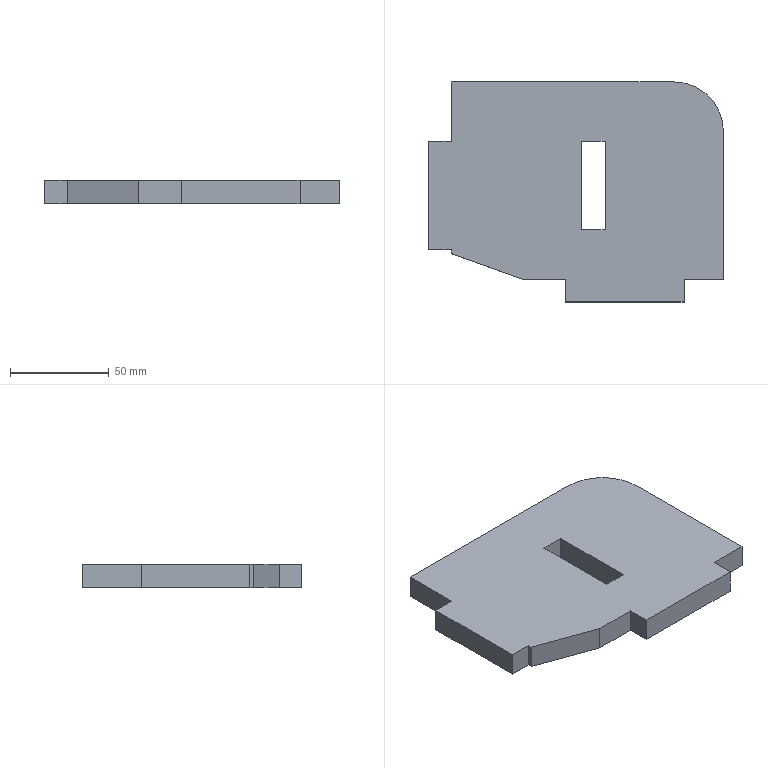Part | SolidWorks | features FlatPattern 1, SMBaseFlange 1, SheetMetal 1 | 1 solid | 20 faces | box 149.5 x 111.5 x 12 mm | volume 170572 mm3 | plane 19 | cylinder 1 | commonest cylinder face diameters 50 x1
STEP:
#1=CARTESIAN_POINT('',(382.937,67.282,0.));
#2=VERTEX_POINT('',#1);
#3=CARTESIAN_POINT('',(382.937,142.282,0.));
#4=VERTEX_POINT('',#3);
#5=CARTESIAN_POINT('',(382.937,67.282,0.));
#6=DIRECTION('',(0.,1.,0.));
#7=VECTOR('',#6,1000.);
#8=LINE('',#5,#7);
#9=EDGE_CURVE('',#2,#4,#8,.T.);
#10=ORIENTED_EDGE('',*,*,#9,.F.);
#11=CARTESIAN_POINT('',(382.937,67.282,-12.));
#12=VERTEX_POINT('',#11);
#13=CARTESIAN_POINT('',(382.937,67.282,-12.));
#14=DIRECTION('',(0.,0.,1.));
#15=VECTOR('',#14,1000.);
#16=LINE('',#13,#15);
#17=EDGE_CURVE('',#12,#2,#16,.T.);
#18=ORIENTED_EDGE('',*,*,#17,.F.);
#19=CARTESIAN_POINT('',(382.937,142.282,-12.));
#20=VERTEX_POINT('',#19);
#21=CARTESIAN_POINT('',(382.937,67.282,-12.));
#22=DIRECTION('',(0.,1.,0.));
#23=VECTOR('',#22,1000.);
#24=LINE('',#21,#23);
#25=EDGE_CURVE('',#12,#20,#24,.T.);
#26=ORIENTED_EDGE('',*,*,#25,.T.);
#27=CARTESIAN_POINT('',(382.937,142.282,-12.));
#28=DIRECTION('',(0.,0.,1.));
#29=VECTOR('',#28,1000.);
#30=LINE('',#27,#29);
#31=EDGE_CURVE('',#20,#4,#30,.T.);
#32=ORIENTED_EDGE('',*,*,#31,.T.);
#33=EDGE_LOOP('',(#10,#18,#26,#32));
#34=FACE_OUTER_BOUND('',#33,.T.);
#35=CARTESIAN_POINT('',(382.937,67.282,-12.));
#36=DIRECTION('',(1.,0.,0.));
#37=DIRECTION('',(0.,0.,-1.));
#38=AXIS2_PLACEMENT_3D('',#35,#36,#37);
#39=PLANE('',#38);
#40=ADVANCED_FACE('',(#34),#39,.T.);
#41=CARTESIAN_POINT('',(362.937,67.282,0.));
#42=VERTEX_POINT('',#41);
#43=CARTESIAN_POINT('',(382.937,67.282,0.));
#44=DIRECTION('',(1.,0.,0.));
#45=VECTOR('',#44,1000.);
#46=LINE('',#43,#45);
#47=EDGE_CURVE('',#42,#2,#46,.T.);
#48=ORIENTED_EDGE('',*,*,#47,.F.);
#49=CARTESIAN_POINT('',(362.937,67.282,-12.));
#50=VERTEX_POINT('',#49);
#51=CARTESIAN_POINT('',(362.937,67.282,-12.));
#52=DIRECTION('',(0.,0.,1.));
#53=VECTOR('',#52,1000.);
#54=LINE('',#51,#53);
#55=EDGE_CURVE('',#50,#42,#54,.T.);
#56=ORIENTED_EDGE('',*,*,#55,.F.);
#57=CARTESIAN_POINT('',(382.937,67.282,-12.));
#58=DIRECTION('',(1.,0.,0.));
#59=VECTOR('',#58,1000.);
#60=LINE('',#57,#59);
#61=EDGE_CURVE('',#50,#12,#60,.T.);
#62=ORIENTED_EDGE('',*,*,#61,.T.);
#63=ORIENTED_EDGE('',*,*,#17,.T.);
#64=EDGE_LOOP('',(#48,#56,#62,#63));
#65=FACE_OUTER_BOUND('',#64,.T.);
#66=CARTESIAN_POINT('',(382.937,67.282,-12.));
#67=DIRECTION('',(0.,-1.,0.));
#68=DIRECTION('',(0.,0.,-1.));
#69=AXIS2_PLACEMENT_3D('',#66,#67,#68);
#70=PLANE('',#69);
#71=ADVANCED_FACE('',(#65),#70,.T.);
#72=CARTESIAN_POINT('',(362.937,55.782,0.));
#73=VERTEX_POINT('',#72);
#74=CARTESIAN_POINT('',(362.937,55.782,0.));
#75=DIRECTION('',(0.,1.,0.));
#76=VECTOR('',#75,1000.);
#77=LINE('',#74,#76);
#78=EDGE_CURVE('',#73,#42,#77,.T.);
#79=ORIENTED_EDGE('',*,*,#78,.F.);
#80=CARTESIAN_POINT('',(362.937,55.782,-12.));
#81=VERTEX_POINT('',#80);
#82=CARTESIAN_POINT('',(362.937,55.782,-12.));
#83=DIRECTION('',(0.,0.,1.));
#84=VECTOR('',#83,1000.);
#85=LINE('',#82,#84);
#86=EDGE_CURVE('',#81,#73,#85,.T.);
#87=ORIENTED_EDGE('',*,*,#86,.F.);
#88=CARTESIAN_POINT('',(362.937,55.782,-12.));
#89=DIRECTION('',(0.,1.,0.));
#90=VECTOR('',#89,1000.);
#91=LINE('',#88,#90);
#92=EDGE_CURVE('',#81,#50,#91,.T.);
#93=ORIENTED_EDGE('',*,*,#92,.T.);
#94=ORIENTED_EDGE('',*,*,#55,.T.);
#95=EDGE_LOOP('',(#79,#87,#93,#94));
#96=FACE_OUTER_BOUND('',#95,.T.);
#97=CARTESIAN_POINT('',(362.937,55.782,-12.));
#98=DIRECTION('',(1.,0.,0.));
#99=DIRECTION('',(0.,0.,-1.));
#100=AXIS2_PLACEMENT_3D('',#97,#98,#99);
#101=PLANE('',#100);
#102=ADVANCED_FACE('',(#96),#101,.T.);
#103=CARTESIAN_POINT('',(302.937,55.782,0.));
#104=VERTEX_POINT('',#103);
#105=CARTESIAN_POINT('',(302.937,55.782,0.));
#106=DIRECTION('',(1.,0.,0.));
#107=VECTOR('',#106,1000.);
#108=LINE('',#105,#107);
#109=EDGE_CURVE('',#104,#73,#108,.T.);
#110=ORIENTED_EDGE('',*,*,#109,.F.);
#111=CARTESIAN_POINT('',(302.937,55.782,-12.));
#112=VERTEX_POINT('',#111);
#113=CARTESIAN_POINT('',(302.937,55.782,-12.));
#114=DIRECTION('',(0.,0.,1.));
#115=VECTOR('',#114,1000.);
#116=LINE('',#113,#115);
#117=EDGE_CURVE('',#112,#104,#116,.T.);
#118=ORIENTED_EDGE('',*,*,#117,.F.);
#119=CARTESIAN_POINT('',(302.937,55.782,-12.));
#120=DIRECTION('',(1.,0.,0.));
#121=VECTOR('',#120,1000.);
#122=LINE('',#119,#121);
#123=EDGE_CURVE('',#112,#81,#122,.T.);
#124=ORIENTED_EDGE('',*,*,#123,.T.);
#125=ORIENTED_EDGE('',*,*,#86,.T.);
#126=EDGE_LOOP('',(#110,#118,#124,#125));
#127=FACE_OUTER_BOUND('',#126,.T.);
#128=CARTESIAN_POINT('',(302.937,55.782,-12.));
#129=DIRECTION('',(0.,-1.,0.));
#130=DIRECTION('',(0.,0.,-1.));
#131=AXIS2_PLACEMENT_3D('',#128,#129,#130);
#132=PLANE('',#131);
#133=ADVANCED_FACE('',(#127),#132,.T.);
#134=CARTESIAN_POINT('',(302.937,67.282,0.));
#135=VERTEX_POINT('',#134);
#136=CARTESIAN_POINT('',(302.937,67.282,0.));
#137=DIRECTION('',(0.,-1.,0.));
#138=VECTOR('',#137,1000.);
#139=LINE('',#136,#138);
#140=EDGE_CURVE('',#135,#104,#139,.T.);
#141=ORIENTED_EDGE('',*,*,#140,.F.);
#142=CARTESIAN_POINT('',(302.937,67.282,-12.));
#143=VERTEX_POINT('',#142);
#144=CARTESIAN_POINT('',(302.937,67.282,-12.));
#145=DIRECTION('',(0.,0.,1.));
#146=VECTOR('',#145,1000.);
#147=LINE('',#144,#146);
#148=EDGE_CURVE('',#143,#135,#147,.T.);
#149=ORIENTED_EDGE('',*,*,#148,.F.);
#150=CARTESIAN_POINT('',(302.937,67.282,-12.));
#151=DIRECTION('',(0.,-1.,0.));
#152=VECTOR('',#151,1000.);
#153=LINE('',#150,#152);
#154=EDGE_CURVE('',#143,#112,#153,.T.);
#155=ORIENTED_EDGE('',*,*,#154,.T.);
#156=ORIENTED_EDGE('',*,*,#117,.T.);
#157=EDGE_LOOP('',(#141,#149,#155,#156));
#158=FACE_OUTER_BOUND('',#157,.T.);
#159=CARTESIAN_POINT('',(302.937,67.282,-12.));
#160=DIRECTION('',(-1.,0.,0.));
#161=DIRECTION('',(0.,0.,1.));
#162=AXIS2_PLACEMENT_3D('',#159,#160,#161);
#163=PLANE('',#162);
#164=ADVANCED_FACE('',(#158),#163,.T.);
#165=CARTESIAN_POINT('',(280.937,67.282,0.));
#166=VERTEX_POINT('',#165);
#167=CARTESIAN_POINT('',(302.937,67.282,0.));
#168=DIRECTION('',(1.,0.,0.));
#169=VECTOR('',#168,1000.);
#170=LINE('',#167,#169);
#171=EDGE_CURVE('',#166,#135,#170,.T.);
#172=ORIENTED_EDGE('',*,*,#171,.F.);
#173=CARTESIAN_POINT('',(280.937,67.282,-12.));
#174=VERTEX_POINT('',#173);
#175=CARTESIAN_POINT('',(280.937,67.282,-12.));
#176=DIRECTION('',(0.,0.,1.));
#177=VECTOR('',#176,1000.);
#178=LINE('',#175,#177);
#179=EDGE_CURVE('',#174,#166,#178,.T.);
#180=ORIENTED_EDGE('',*,*,#179,.F.);
#181=CARTESIAN_POINT('',(302.937,67.282,-12.));
#182=DIRECTION('',(1.,0.,0.));
#183=VECTOR('',#182,1000.);
#184=LINE('',#181,#183);
#185=EDGE_CURVE('',#174,#143,#184,.T.);
#186=ORIENTED_EDGE('',*,*,#185,.T.);
#187=ORIENTED_EDGE('',*,*,#148,.T.);
#188=EDGE_LOOP('',(#172,#180,#186,#187));
#189=FACE_OUTER_BOUND('',#188,.T.);
#190=CARTESIAN_POINT('',(302.937,67.282,-12.));
#191=DIRECTION('',(0.,-1.,0.));
#192=DIRECTION('',(1.,0.,0.));
#193=AXIS2_PLACEMENT_3D('',#190,#191,#192);
#194=PLANE('',#193);
#195=ADVANCED_FACE('',(#189),#194,.T.);
#196=CARTESIAN_POINT('',(244.937,80.282,0.));
#197=VERTEX_POINT('',#196);
#198=CARTESIAN_POINT('',(280.937,67.282,0.));
#199=DIRECTION('',(0.9406,-0.3396,0.));
#200=VECTOR('',#199,1000.);
#201=LINE('',#198,#200);
#202=EDGE_CURVE('',#197,#166,#201,.T.);
#203=ORIENTED_EDGE('',*,*,#202,.F.);
#204=CARTESIAN_POINT('',(244.937,80.282,-12.));
#205=VERTEX_POINT('',#204);
#206=CARTESIAN_POINT('',(244.937,80.282,-12.));
#207=DIRECTION('',(0.,0.,1.));
#208=VECTOR('',#207,1000.);
#209=LINE('',#206,#208);
#210=EDGE_CURVE('',#205,#197,#209,.T.);
#211=ORIENTED_EDGE('',*,*,#210,.F.);
#212=CARTESIAN_POINT('',(280.937,67.282,-12.));
#213=DIRECTION('',(0.9406,-0.3396,0.));
#214=VECTOR('',#213,1000.);
#215=LINE('',#212,#214);
#216=EDGE_CURVE('',#205,#174,#215,.T.);
#217=ORIENTED_EDGE('',*,*,#216,.T.);
#218=ORIENTED_EDGE('',*,*,#179,.T.);
#219=EDGE_LOOP('',(#203,#211,#217,#218));
#220=FACE_OUTER_BOUND('',#219,.T.);
#221=CARTESIAN_POINT('',(280.937,67.282,-12.));
#222=DIRECTION('',(-0.3396,-0.9406,0.));
#223=DIRECTION('',(0.9406,-0.3396,0.));
#224=AXIS2_PLACEMENT_3D('',#221,#222,#223);
#225=PLANE('',#224);
#226=ADVANCED_FACE('',(#220),#225,.T.);
#227=CARTESIAN_POINT('',(244.937,82.282,0.));
#228=VERTEX_POINT('',#227);
#229=CARTESIAN_POINT('',(244.937,80.282,0.));
#230=DIRECTION('',(0.,-1.,0.));
#231=VECTOR('',#230,1000.);
#232=LINE('',#229,#231);
#233=EDGE_CURVE('',#228,#197,#232,.T.);
#234=ORIENTED_EDGE('',*,*,#233,.F.);
#235=CARTESIAN_POINT('',(244.937,82.282,-12.));
#236=VERTEX_POINT('',#235);
#237=CARTESIAN_POINT('',(244.937,82.282,-12.));
#238=DIRECTION('',(0.,0.,1.));
#239=VECTOR('',#238,1000.);
#240=LINE('',#237,#239);
#241=EDGE_CURVE('',#236,#228,#240,.T.);
#242=ORIENTED_EDGE('',*,*,#241,.F.);
#243=CARTESIAN_POINT('',(244.937,80.282,-12.));
#244=DIRECTION('',(0.,-1.,0.));
#245=VECTOR('',#244,1000.);
#246=LINE('',#243,#245);
#247=EDGE_CURVE('',#236,#205,#246,.T.);
#248=ORIENTED_EDGE('',*,*,#247,.T.);
#249=ORIENTED_EDGE('',*,*,#210,.T.);
#250=EDGE_LOOP('',(#234,#242,#248,#249));
#251=FACE_OUTER_BOUND('',#250,.T.);
#252=CARTESIAN_POINT('',(244.937,80.282,-12.));
#253=DIRECTION('',(-1.,0.,0.));
#254=DIRECTION('',(0.,-1.,0.));
#255=AXIS2_PLACEMENT_3D('',#252,#253,#254);
#256=PLANE('',#255);
#257=ADVANCED_FACE('',(#251),#256,.T.);
#258=CARTESIAN_POINT('',(233.437,82.282,0.));
#259=VERTEX_POINT('',#258);
#260=CARTESIAN_POINT('',(233.437,82.282,0.));
#261=DIRECTION('',(1.,0.,0.));
#262=VECTOR('',#261,1000.);
#263=LINE('',#260,#262);
#264=EDGE_CURVE('',#259,#228,#263,.T.);
#265=ORIENTED_EDGE('',*,*,#264,.F.);
#266=CARTESIAN_POINT('',(233.437,82.282,-12.));
#267=VERTEX_POINT('',#266);
#268=CARTESIAN_POINT('',(233.437,82.282,-12.));
#269=DIRECTION('',(0.,0.,1.));
#270=VECTOR('',#269,1000.);
#271=LINE('',#268,#270);
#272=EDGE_CURVE('',#267,#259,#271,.T.);
#273=ORIENTED_EDGE('',*,*,#272,.F.);
#274=CARTESIAN_POINT('',(233.437,82.282,-12.));
#275=DIRECTION('',(1.,0.,0.));
#276=VECTOR('',#275,1000.);
#277=LINE('',#274,#276);
#278=EDGE_CURVE('',#267,#236,#277,.T.);
#279=ORIENTED_EDGE('',*,*,#278,.T.);
#280=ORIENTED_EDGE('',*,*,#241,.T.);
#281=EDGE_LOOP('',(#265,#273,#279,#280));
#282=FACE_OUTER_BOUND('',#281,.T.);
#283=CARTESIAN_POINT('',(233.437,82.282,-12.));
#284=DIRECTION('',(0.,-1.,0.));
#285=DIRECTION('',(0.,0.,-1.));
#286=AXIS2_PLACEMENT_3D('',#283,#284,#285);
#287=PLANE('',#286);
#288=ADVANCED_FACE('',(#282),#287,.T.);
#289=CARTESIAN_POINT('',(233.437,137.282,0.));
#290=VERTEX_POINT('',#289);
#291=CARTESIAN_POINT('',(233.437,137.282,0.));
#292=DIRECTION('',(0.,-1.,0.));
#293=VECTOR('',#292,1000.);
#294=LINE('',#291,#293);
#295=EDGE_CURVE('',#290,#259,#294,.T.);
#296=ORIENTED_EDGE('',*,*,#295,.F.);
#297=CARTESIAN_POINT('',(233.437,137.282,-12.));
#298=VERTEX_POINT('',#297);
#299=CARTESIAN_POINT('',(233.437,137.282,-12.));
#300=DIRECTION('',(0.,0.,1.));
#301=VECTOR('',#300,1000.);
#302=LINE('',#299,#301);
#303=EDGE_CURVE('',#298,#290,#302,.T.);
#304=ORIENTED_EDGE('',*,*,#303,.F.);
#305=CARTESIAN_POINT('',(233.437,137.282,-12.));
#306=DIRECTION('',(0.,-1.,0.));
#307=VECTOR('',#306,1000.);
#308=LINE('',#305,#307);
#309=EDGE_CURVE('',#298,#267,#308,.T.);
#310=ORIENTED_EDGE('',*,*,#309,.T.);
#311=ORIENTED_EDGE('',*,*,#272,.T.);
#312=EDGE_LOOP('',(#296,#304,#310,#311));
#313=FACE_OUTER_BOUND('',#312,.T.);
#314=CARTESIAN_POINT('',(233.437,137.282,-12.));
#315=DIRECTION('',(-1.,0.,0.));
#316=DIRECTION('',(0.,0.,1.));
#317=AXIS2_PLACEMENT_3D('',#314,#315,#316);
#318=PLANE('',#317);
#319=ADVANCED_FACE('',(#313),#318,.T.);
#320=CARTESIAN_POINT('',(244.937,137.282,0.));
#321=VERTEX_POINT('',#320);
#322=CARTESIAN_POINT('',(244.937,137.282,0.));
#323=DIRECTION('',(-1.,0.,0.));
#324=VECTOR('',#323,1000.);
#325=LINE('',#322,#324);
#326=EDGE_CURVE('',#321,#290,#325,.T.);
#327=ORIENTED_EDGE('',*,*,#326,.F.);
#328=CARTESIAN_POINT('',(244.937,137.282,-12.));
#329=VERTEX_POINT('',#328);
#330=CARTESIAN_POINT('',(244.937,137.282,-12.));
#331=DIRECTION('',(0.,0.,1.));
#332=VECTOR('',#331,1000.);
#333=LINE('',#330,#332);
#334=EDGE_CURVE('',#329,#321,#333,.T.);
#335=ORIENTED_EDGE('',*,*,#334,.F.);
#336=CARTESIAN_POINT('',(244.937,137.282,-12.));
#337=DIRECTION('',(-1.,0.,0.));
#338=VECTOR('',#337,1000.);
#339=LINE('',#336,#338);
#340=EDGE_CURVE('',#329,#298,#339,.T.);
#341=ORIENTED_EDGE('',*,*,#340,.T.);
#342=ORIENTED_EDGE('',*,*,#303,.T.);
#343=EDGE_LOOP('',(#327,#335,#341,#342));
#344=FACE_OUTER_BOUND('',#343,.T.);
#345=CARTESIAN_POINT('',(244.937,137.282,-12.));
#346=DIRECTION('',(0.,1.,0.));
#347=DIRECTION('',(0.,0.,1.));
#348=AXIS2_PLACEMENT_3D('',#345,#346,#347);
#349=PLANE('',#348);
#350=ADVANCED_FACE('',(#344),#349,.T.);
#351=CARTESIAN_POINT('',(244.937,167.282,0.));
#352=VERTEX_POINT('',#351);
#353=CARTESIAN_POINT('',(244.937,137.282,0.));
#354=DIRECTION('',(0.,-1.,0.));
#355=VECTOR('',#354,1000.);
#356=LINE('',#353,#355);
#357=EDGE_CURVE('',#352,#321,#356,.T.);
#358=ORIENTED_EDGE('',*,*,#357,.F.);
#359=CARTESIAN_POINT('',(244.937,167.282,-12.));
#360=VERTEX_POINT('',#359);
#361=CARTESIAN_POINT('',(244.937,167.282,-12.));
#362=DIRECTION('',(0.,0.,1.));
#363=VECTOR('',#362,1000.);
#364=LINE('',#361,#363);
#365=EDGE_CURVE('',#360,#352,#364,.T.);
#366=ORIENTED_EDGE('',*,*,#365,.F.);
#367=CARTESIAN_POINT('',(244.937,137.282,-12.));
#368=DIRECTION('',(0.,-1.,0.));
#369=VECTOR('',#368,1000.);
#370=LINE('',#367,#369);
#371=EDGE_CURVE('',#360,#329,#370,.T.);
#372=ORIENTED_EDGE('',*,*,#371,.T.);
#373=ORIENTED_EDGE('',*,*,#334,.T.);
#374=EDGE_LOOP('',(#358,#366,#372,#373));
#375=FACE_OUTER_BOUND('',#374,.T.);
#376=CARTESIAN_POINT('',(244.937,137.282,-12.));
#377=DIRECTION('',(-1.,0.,0.));
#378=DIRECTION('',(0.,-1.,0.));
#379=AXIS2_PLACEMENT_3D('',#376,#377,#378);
#380=PLANE('',#379);
#381=ADVANCED_FACE('',(#375),#380,.T.);
#382=CARTESIAN_POINT('',(357.937,167.282,0.));
#383=VERTEX_POINT('',#382);
#384=CARTESIAN_POINT('',(357.937,167.282,0.));
#385=DIRECTION('',(-1.,0.,0.));
#386=VECTOR('',#385,1000.);
#387=LINE('',#384,#386);
#388=EDGE_CURVE('',#383,#352,#387,.T.);
#389=ORIENTED_EDGE('',*,*,#388,.F.);
#390=CARTESIAN_POINT('',(357.937,167.282,-12.));
#391=VERTEX_POINT('',#390);
#392=CARTESIAN_POINT('',(357.937,167.282,-12.));
#393=DIRECTION('',(0.,0.,1.));
#394=VECTOR('',#393,1000.);
#395=LINE('',#392,#394);
#396=EDGE_CURVE('',#391,#383,#395,.T.);
#397=ORIENTED_EDGE('',*,*,#396,.F.);
#398=CARTESIAN_POINT('',(357.937,167.282,-12.));
#399=DIRECTION('',(-1.,0.,0.));
#400=VECTOR('',#399,1000.);
#401=LINE('',#398,#400);
#402=EDGE_CURVE('',#391,#360,#401,.T.);
#403=ORIENTED_EDGE('',*,*,#402,.T.);
#404=ORIENTED_EDGE('',*,*,#365,.T.);
#405=EDGE_LOOP('',(#389,#397,#403,#404));
#406=FACE_OUTER_BOUND('',#405,.T.);
#407=CARTESIAN_POINT('',(357.937,167.282,-12.));
#408=DIRECTION('',(0.,1.,0.));
#409=DIRECTION('',(-1.,0.,0.));
#410=AXIS2_PLACEMENT_3D('',#407,#408,#409);
#411=PLANE('',#410);
#412=ADVANCED_FACE('',(#406),#411,.T.);
#413=CARTESIAN_POINT('',(357.937,142.282,0.));
#414=DIRECTION('',(0.,0.,1.));
#415=DIRECTION('',(1.,0.,0.));
#416=AXIS2_PLACEMENT_3D('',#413,#414,#415);
#417=CIRCLE('',#416,25.);
#418=EDGE_CURVE('',#4,#383,#417,.T.);
#419=ORIENTED_EDGE('',*,*,#418,.F.);
#420=ORIENTED_EDGE('',*,*,#31,.F.);
#421=CARTESIAN_POINT('',(357.937,142.282,-12.));
#422=DIRECTION('',(0.,0.,1.));
#423=DIRECTION('',(1.,0.,0.));
#424=AXIS2_PLACEMENT_3D('',#421,#422,#423);
#425=CIRCLE('',#424,25.);
#426=EDGE_CURVE('',#20,#391,#425,.T.);
#427=ORIENTED_EDGE('',*,*,#426,.T.);
#428=ORIENTED_EDGE('',*,*,#396,.T.);
#429=EDGE_LOOP('',(#419,#420,#427,#428));
#430=FACE_OUTER_BOUND('',#429,.T.);
#431=CARTESIAN_POINT('',(357.937,142.282,-12.));
#432=DIRECTION('',(0.,0.,1.));
#433=DIRECTION('',(1.,0.,0.));
#434=AXIS2_PLACEMENT_3D('',#431,#432,#433);
#435=CYLINDRICAL_SURFACE('',#434,25.);
#436=ADVANCED_FACE('',(#430),#435,.T.);
#437=CARTESIAN_POINT('',(310.937,92.282,-12.));
#438=VERTEX_POINT('',#437);
#439=CARTESIAN_POINT('',(322.937,92.282,-12.));
#440=VERTEX_POINT('',#439);
#441=CARTESIAN_POINT('',(322.937,92.282,-12.));
#442=DIRECTION('',(1.,0.,0.));
#443=VECTOR('',#442,1000.);
#444=LINE('',#441,#443);
#445=EDGE_CURVE('',#438,#440,#444,.T.);
#446=ORIENTED_EDGE('',*,*,#445,.T.);
#447=CARTESIAN_POINT('',(322.937,137.282,-12.));
#448=VERTEX_POINT('',#447);
#449=CARTESIAN_POINT('',(322.937,137.282,-12.));
#450=DIRECTION('',(0.,1.,0.));
#451=VECTOR('',#450,1000.);
#452=LINE('',#449,#451);
#453=EDGE_CURVE('',#440,#448,#452,.T.);
#454=ORIENTED_EDGE('',*,*,#453,.T.);
#455=CARTESIAN_POINT('',(310.937,137.282,-12.));
#456=VERTEX_POINT('',#455);
#457=CARTESIAN_POINT('',(322.937,137.282,-12.));
#458=DIRECTION('',(-1.,0.,0.));
#459=VECTOR('',#458,1000.);
#460=LINE('',#457,#459);
#461=EDGE_CURVE('',#448,#456,#460,.T.);
#462=ORIENTED_EDGE('',*,*,#461,.T.);
#463=CARTESIAN_POINT('',(310.937,137.282,-12.));
#464=DIRECTION('',(0.,-1.,0.));
#465=VECTOR('',#464,1000.);
#466=LINE('',#463,#465);
#467=EDGE_CURVE('',#456,#438,#466,.T.);
#468=ORIENTED_EDGE('',*,*,#467,.T.);
#469=EDGE_LOOP('',(#446,#454,#462,#468));
#470=FACE_BOUND('',#469,.T.);
#471=ORIENTED_EDGE('',*,*,#25,.F.);
#472=ORIENTED_EDGE('',*,*,#61,.F.);
#473=ORIENTED_EDGE('',*,*,#92,.F.);
#474=ORIENTED_EDGE('',*,*,#123,.F.);
#475=ORIENTED_EDGE('',*,*,#154,.F.);
#476=ORIENTED_EDGE('',*,*,#185,.F.);
#477=ORIENTED_EDGE('',*,*,#216,.F.);
#478=ORIENTED_EDGE('',*,*,#247,.F.);
#479=ORIENTED_EDGE('',*,*,#278,.F.);
#480=ORIENTED_EDGE('',*,*,#309,.F.);
#481=ORIENTED_EDGE('',*,*,#340,.F.);
#482=ORIENTED_EDGE('',*,*,#371,.F.);
#483=ORIENTED_EDGE('',*,*,#402,.F.);
#484=ORIENTED_EDGE('',*,*,#426,.F.);
#485=EDGE_LOOP('',(#471,#472,#473,#474,#475,#476,#477,#478,#479,#480,#481,#482,#483,#484));
#486=FACE_OUTER_BOUND('',#485,.T.);
#487=CARTESIAN_POINT('',(357.937,142.282,-12.));
#488=DIRECTION('',(0.,0.,1.));
#489=DIRECTION('',(1.,0.,0.));
#490=AXIS2_PLACEMENT_3D('',#487,#488,#489);
#491=PLANE('',#490);
#492=ADVANCED_FACE('',(#470,#486),#491,.F.);
#493=CARTESIAN_POINT('',(322.937,92.282,0.));
#494=VERTEX_POINT('',#493);
#495=CARTESIAN_POINT('',(322.937,137.282,0.));
#496=VERTEX_POINT('',#495);
#497=CARTESIAN_POINT('',(322.937,137.282,0.));
#498=DIRECTION('',(0.,1.,0.));
#499=VECTOR('',#498,1000.);
#500=LINE('',#497,#499);
#501=EDGE_CURVE('',#494,#496,#500,.T.);
#502=ORIENTED_EDGE('',*,*,#501,.F.);
#503=CARTESIAN_POINT('',(310.937,92.282,0.));
#504=VERTEX_POINT('',#503);
#505=CARTESIAN_POINT('',(322.937,92.282,0.));
#506=DIRECTION('',(1.,0.,0.));
#507=VECTOR('',#506,1000.);
#508=LINE('',#505,#507);
#509=EDGE_CURVE('',#504,#494,#508,.T.);
#510=ORIENTED_EDGE('',*,*,#509,.F.);
#511=CARTESIAN_POINT('',(310.937,137.282,0.));
#512=VERTEX_POINT('',#511);
#513=CARTESIAN_POINT('',(310.937,137.282,0.));
#514=DIRECTION('',(0.,-1.,0.));
#515=VECTOR('',#514,1000.);
#516=LINE('',#513,#515);
#517=EDGE_CURVE('',#512,#504,#516,.T.);
#518=ORIENTED_EDGE('',*,*,#517,.F.);
#519=CARTESIAN_POINT('',(322.937,137.282,0.));
#520=DIRECTION('',(-1.,0.,0.));
#521=VECTOR('',#520,1000.);
#522=LINE('',#519,#521);
#523=EDGE_CURVE('',#496,#512,#522,.T.);
#524=ORIENTED_EDGE('',*,*,#523,.F.);
#525=EDGE_LOOP('',(#502,#510,#518,#524));
#526=FACE_BOUND('',#525,.T.);
#527=ORIENTED_EDGE('',*,*,#9,.T.);
#528=ORIENTED_EDGE('',*,*,#418,.T.);
#529=ORIENTED_EDGE('',*,*,#388,.T.);
#530=ORIENTED_EDGE('',*,*,#357,.T.);
#531=ORIENTED_EDGE('',*,*,#326,.T.);
#532=ORIENTED_EDGE('',*,*,#295,.T.);
#533=ORIENTED_EDGE('',*,*,#264,.T.);
#534=ORIENTED_EDGE('',*,*,#233,.T.);
#535=ORIENTED_EDGE('',*,*,#202,.T.);
#536=ORIENTED_EDGE('',*,*,#171,.T.);
#537=ORIENTED_EDGE('',*,*,#140,.T.);
#538=ORIENTED_EDGE('',*,*,#109,.T.);
#539=ORIENTED_EDGE('',*,*,#78,.T.);
#540=ORIENTED_EDGE('',*,*,#47,.T.);
#541=EDGE_LOOP('',(#527,#528,#529,#530,#531,#532,#533,#534,#535,#536,#537,#538,#539,#540));
#542=FACE_OUTER_BOUND('',#541,.T.);
#543=CARTESIAN_POINT('',(357.937,142.282,0.));
#544=DIRECTION('',(0.,0.,1.));
#545=DIRECTION('',(1.,0.,0.));
#546=AXIS2_PLACEMENT_3D('',#543,#544,#545);
#547=PLANE('',#546);
#548=ADVANCED_FACE('',(#526,#542),#547,.T.);
#549=ORIENTED_EDGE('',*,*,#501,.T.);
#550=CARTESIAN_POINT('',(322.937,137.282,-12.));
#551=DIRECTION('',(0.,0.,1.));
#552=VECTOR('',#551,1000.);
#553=LINE('',#550,#552);
#554=EDGE_CURVE('',#448,#496,#553,.T.);
#555=ORIENTED_EDGE('',*,*,#554,.F.);
#556=ORIENTED_EDGE('',*,*,#453,.F.);
#557=CARTESIAN_POINT('',(322.937,92.282,-12.));
#558=DIRECTION('',(0.,0.,1.));
#559=VECTOR('',#558,1000.);
#560=LINE('',#557,#559);
#561=EDGE_CURVE('',#440,#494,#560,.T.);
#562=ORIENTED_EDGE('',*,*,#561,.T.);
#563=EDGE_LOOP('',(#549,#555,#556,#562));
#564=FACE_OUTER_BOUND('',#563,.T.);
#565=CARTESIAN_POINT('',(322.937,137.282,-12.));
#566=DIRECTION('',(1.,0.,0.));
#567=DIRECTION('',(0.,0.,-1.));
#568=AXIS2_PLACEMENT_3D('',#565,#566,#567);
#569=PLANE('',#568);
#570=ADVANCED_FACE('',(#564),#569,.F.);
#571=ORIENTED_EDGE('',*,*,#509,.T.);
#572=ORIENTED_EDGE('',*,*,#561,.F.);
#573=ORIENTED_EDGE('',*,*,#445,.F.);
#574=CARTESIAN_POINT('',(310.937,92.282,-12.));
#575=DIRECTION('',(0.,0.,1.));
#576=VECTOR('',#575,1000.);
#577=LINE('',#574,#576);
#578=EDGE_CURVE('',#438,#504,#577,.T.);
#579=ORIENTED_EDGE('',*,*,#578,.T.);
#580=EDGE_LOOP('',(#571,#572,#573,#579));
#581=FACE_OUTER_BOUND('',#580,.T.);
#582=CARTESIAN_POINT('',(322.937,92.282,-12.));
#583=DIRECTION('',(0.,-1.,0.));
#584=DIRECTION('',(0.,0.,-1.));
#585=AXIS2_PLACEMENT_3D('',#582,#583,#584);
#586=PLANE('',#585);
#587=ADVANCED_FACE('',(#581),#586,.F.);
#588=ORIENTED_EDGE('',*,*,#517,.T.);
#589=ORIENTED_EDGE('',*,*,#578,.F.);
#590=ORIENTED_EDGE('',*,*,#467,.F.);
#591=CARTESIAN_POINT('',(310.937,137.282,-12.));
#592=DIRECTION('',(0.,0.,1.));
#593=VECTOR('',#592,1000.);
#594=LINE('',#591,#593);
#595=EDGE_CURVE('',#456,#512,#594,.T.);
#596=ORIENTED_EDGE('',*,*,#595,.T.);
#597=EDGE_LOOP('',(#588,#589,#590,#596));
#598=FACE_OUTER_BOUND('',#597,.T.);
#599=CARTESIAN_POINT('',(310.937,137.282,-12.));
#600=DIRECTION('',(-1.,0.,0.));
#601=DIRECTION('',(0.,0.,1.));
#602=AXIS2_PLACEMENT_3D('',#599,#600,#601);
#603=PLANE('',#602);
#604=ADVANCED_FACE('',(#598),#603,.F.);
#605=ORIENTED_EDGE('',*,*,#523,.T.);
#606=ORIENTED_EDGE('',*,*,#595,.F.);
#607=ORIENTED_EDGE('',*,*,#461,.F.);
#608=ORIENTED_EDGE('',*,*,#554,.T.);
#609=EDGE_LOOP('',(#605,#606,#607,#608));
#610=FACE_OUTER_BOUND('',#609,.T.);
#611=CARTESIAN_POINT('',(322.937,137.282,-12.));
#612=DIRECTION('',(0.,1.,0.));
#613=DIRECTION('',(0.,0.,1.));
#614=AXIS2_PLACEMENT_3D('',#611,#612,#613);
#615=PLANE('',#614);
#616=ADVANCED_FACE('',(#610),#615,.F.);
#617=CLOSED_SHELL('',(#40,#71,#102,#133,#164,#195,#226,#257,#288,#319,#350,#381,#412,#436,#492,#548,#570,#587,#604,#616));
#618=MANIFOLD_SOLID_BREP('',#617);
#619=CARTESIAN_POINT('',(0.,0.,0.));
#620=DIRECTION('',(0.,0.,1.));
#621=DIRECTION('',(1.,0.,0.));
#622=AXIS2_PLACEMENT_3D('',#619,#620,#621);
#623=(LENGTH_UNIT()NAMED_UNIT(*)SI_UNIT(.MILLI.,.METRE.));
#624=UNCERTAINTY_MEASURE_WITH_UNIT(LENGTH_MEASURE(0.00001),#623,'','');
#625=(NAMED_UNIT(*)PLANE_ANGLE_UNIT()SI_UNIT($,.RADIAN.));
#626=(NAMED_UNIT(*)SI_UNIT($,.STERADIAN.)SOLID_ANGLE_UNIT());
#627=(GEOMETRIC_REPRESENTATION_CONTEXT(3)GLOBAL_UNCERTAINTY_ASSIGNED_CONTEXT((#624))GLOBAL_UNIT_ASSIGNED_CONTEXT((#623,#625,#626))REPRESENTATION_CONTEXT('',''));
#628=ADVANCED_BREP_SHAPE_REPRESENTATION('',(#618,#622),#627);